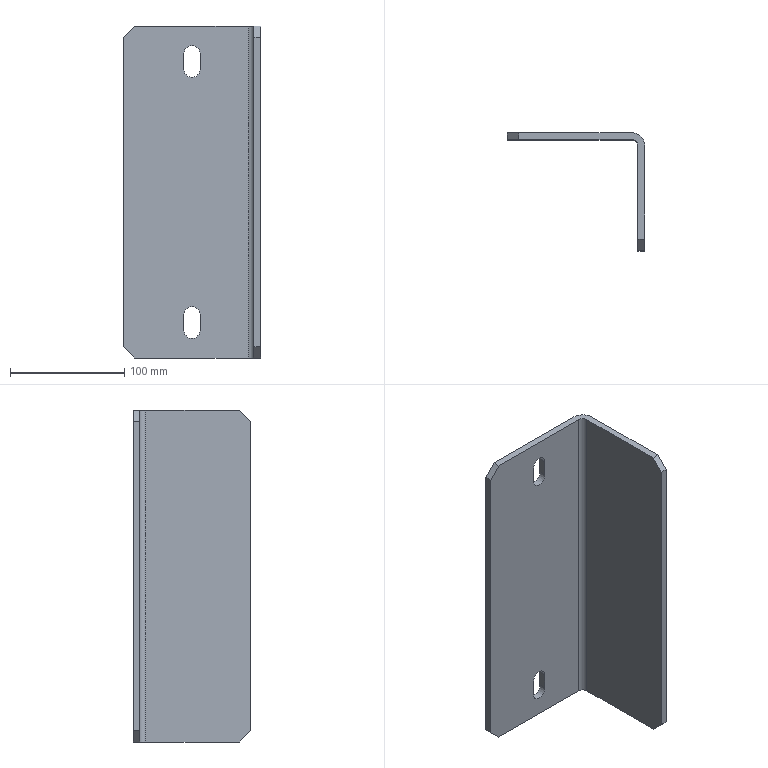Part | STEP file | VD-SYL0380DJ1006_1_1_4-2_VD-SYL | 1 solid | 24 faces | box 120 x 103 x 290 mm | volume 366206 mm3 | plane 16 | cylinder 8 | commonest cylinder face diameters 14 x6 10 x1 22 x1
STEP:
#1=CARTESIAN_POINT('',(7.,22.5,-107.));
#2=VERTEX_POINT('',#1);
#3=CARTESIAN_POINT('',(7.,22.5,-121.));
#4=VERTEX_POINT('',#3);
#5=CARTESIAN_POINT('',(7.,22.5,-107.));
#6=DIRECTION('',(0.,0.,-1.));
#7=VECTOR('',#6,1000.);
#8=LINE('',#5,#7);
#9=EDGE_CURVE('',#2,#4,#8,.T.);
#10=ORIENTED_EDGE('',*,*,#9,.T.);
#11=CARTESIAN_POINT('',(7.,16.5,-121.));
#12=VERTEX_POINT('',#11);
#13=CARTESIAN_POINT('',(7.,16.5,-121.));
#14=DIRECTION('',(0.,1.,0.));
#15=VECTOR('',#14,1000.);
#16=LINE('',#13,#15);
#17=EDGE_CURVE('',#12,#4,#16,.T.);
#18=ORIENTED_EDGE('',*,*,#17,.F.);
#19=CARTESIAN_POINT('',(7.,16.5,-107.));
#20=VERTEX_POINT('',#19);
#21=CARTESIAN_POINT('',(7.,16.5,-107.));
#22=DIRECTION('',(0.,0.,-1.));
#23=VECTOR('',#22,1000.);
#24=LINE('',#21,#23);
#25=EDGE_CURVE('',#20,#12,#24,.T.);
#26=ORIENTED_EDGE('',*,*,#25,.F.);
#27=CARTESIAN_POINT('',(7.,22.5,-107.));
#28=DIRECTION('',(0.,-1.,0.));
#29=VECTOR('',#28,1000.);
#30=LINE('',#27,#29);
#31=EDGE_CURVE('',#2,#20,#30,.T.);
#32=ORIENTED_EDGE('',*,*,#31,.F.);
#33=EDGE_LOOP('',(#10,#18,#26,#32));
#34=FACE_OUTER_BOUND('',#33,.T.);
#35=CARTESIAN_POINT('',(7.,19.5,-117.5));
#36=DIRECTION('',(-1.,0.,0.));
#37=DIRECTION('',(0.,0.,1.));
#38=AXIS2_PLACEMENT_3D('',#35,#36,#37);
#39=PLANE('',#38);
#40=ADVANCED_FACE('',(#34),#39,.T.);
#41=CARTESIAN_POINT('',(0.,22.5,-100.));
#42=VERTEX_POINT('',#41);
#43=CARTESIAN_POINT('',(0.,16.5,-100.));
#44=VERTEX_POINT('',#43);
#45=CARTESIAN_POINT('',(0.,22.5,-100.));
#46=DIRECTION('',(0.,-1.,0.));
#47=VECTOR('',#46,1000.);
#48=LINE('',#45,#47);
#49=EDGE_CURVE('',#42,#44,#48,.T.);
#50=ORIENTED_EDGE('',*,*,#49,.F.);
#51=CARTESIAN_POINT('',(0.,22.5,-107.));
#52=DIRECTION('',(0.,-1.,0.));
#53=DIRECTION('',(1.,0.,0.));
#54=AXIS2_PLACEMENT_3D('',#51,#52,#53);
#55=CIRCLE('',#54,7.);
#56=EDGE_CURVE('',#2,#42,#55,.T.);
#57=ORIENTED_EDGE('',*,*,#56,.F.);
#58=ORIENTED_EDGE('',*,*,#31,.T.);
#59=CARTESIAN_POINT('',(0.,16.5,-107.));
#60=DIRECTION('',(0.,1.,0.));
#61=DIRECTION('',(0.,0.,1.));
#62=AXIS2_PLACEMENT_3D('',#59,#60,#61);
#63=CIRCLE('',#62,7.);
#64=EDGE_CURVE('',#44,#20,#63,.T.);
#65=ORIENTED_EDGE('',*,*,#64,.F.);
#66=EDGE_LOOP('',(#50,#57,#58,#65));
#67=FACE_OUTER_BOUND('',#66,.T.);
#68=CARTESIAN_POINT('',(0.,19.5,-107.));
#69=DIRECTION('',(0.,1.,0.));
#70=DIRECTION('',(0.,0.,1.));
#71=AXIS2_PLACEMENT_3D('',#68,#69,#70);
#72=CYLINDRICAL_SURFACE('',#71,7.);
#73=ADVANCED_FACE('',(#67),#72,.F.);
#74=CARTESIAN_POINT('',(-7.,16.5,-107.));
#75=VERTEX_POINT('',#74);
#76=CARTESIAN_POINT('',(0.,16.5,-107.));
#77=DIRECTION('',(0.,1.,0.));
#78=DIRECTION('',(-1.,0.,0.));
#79=AXIS2_PLACEMENT_3D('',#76,#77,#78);
#80=CIRCLE('',#79,7.);
#81=EDGE_CURVE('',#75,#44,#80,.T.);
#82=ORIENTED_EDGE('',*,*,#81,.F.);
#83=CARTESIAN_POINT('',(-7.,22.5,-107.));
#84=VERTEX_POINT('',#83);
#85=CARTESIAN_POINT('',(-7.,16.5,-107.));
#86=DIRECTION('',(0.,1.,0.));
#87=VECTOR('',#86,1000.);
#88=LINE('',#85,#87);
#89=EDGE_CURVE('',#75,#84,#88,.T.);
#90=ORIENTED_EDGE('',*,*,#89,.T.);
#91=CARTESIAN_POINT('',(0.,22.5,-107.));
#92=DIRECTION('',(0.,-1.,0.));
#93=DIRECTION('',(0.,0.,1.));
#94=AXIS2_PLACEMENT_3D('',#91,#92,#93);
#95=CIRCLE('',#94,7.);
#96=EDGE_CURVE('',#42,#84,#95,.T.);
#97=ORIENTED_EDGE('',*,*,#96,.F.);
#98=ORIENTED_EDGE('',*,*,#49,.T.);
#99=EDGE_LOOP('',(#82,#90,#97,#98));
#100=FACE_OUTER_BOUND('',#99,.T.);
#101=CARTESIAN_POINT('',(0.,19.5,-107.));
#102=DIRECTION('',(0.,1.,0.));
#103=DIRECTION('',(0.,0.,1.));
#104=AXIS2_PLACEMENT_3D('',#101,#102,#103);
#105=CYLINDRICAL_SURFACE('',#104,7.);
#106=ADVANCED_FACE('',(#100),#105,.F.);
#107=CARTESIAN_POINT('',(-7.,22.5,-121.));
#108=VERTEX_POINT('',#107);
#109=CARTESIAN_POINT('',(-7.,22.5,-121.));
#110=DIRECTION('',(0.,0.,1.));
#111=VECTOR('',#110,1000.);
#112=LINE('',#109,#111);
#113=EDGE_CURVE('',#108,#84,#112,.T.);
#114=ORIENTED_EDGE('',*,*,#113,.T.);
#115=ORIENTED_EDGE('',*,*,#89,.F.);
#116=CARTESIAN_POINT('',(-7.,16.5,-121.));
#117=VERTEX_POINT('',#116);
#118=CARTESIAN_POINT('',(-7.,16.5,-121.));
#119=DIRECTION('',(0.,0.,1.));
#120=VECTOR('',#119,1000.);
#121=LINE('',#118,#120);
#122=EDGE_CURVE('',#117,#75,#121,.T.);
#123=ORIENTED_EDGE('',*,*,#122,.F.);
#124=CARTESIAN_POINT('',(-7.,22.5,-121.));
#125=DIRECTION('',(0.,-1.,0.));
#126=VECTOR('',#125,1000.);
#127=LINE('',#124,#126);
#128=EDGE_CURVE('',#108,#117,#127,.T.);
#129=ORIENTED_EDGE('',*,*,#128,.F.);
#130=EDGE_LOOP('',(#114,#115,#123,#129));
#131=FACE_OUTER_BOUND('',#130,.T.);
#132=CARTESIAN_POINT('',(-7.,19.5,-110.5));
#133=DIRECTION('',(1.,0.,0.));
#134=DIRECTION('',(0.,1.,0.));
#135=AXIS2_PLACEMENT_3D('',#132,#133,#134);
#136=PLANE('',#135);
#137=ADVANCED_FACE('',(#131),#136,.T.);
#138=CARTESIAN_POINT('',(-7.,16.5,121.));
#139=VERTEX_POINT('',#138);
#140=CARTESIAN_POINT('',(0.,16.5,128.));
#141=VERTEX_POINT('',#140);
#142=CARTESIAN_POINT('',(0.,16.5,121.));
#143=DIRECTION('',(0.,1.,0.));
#144=DIRECTION('',(-1.,0.,0.));
#145=AXIS2_PLACEMENT_3D('',#142,#143,#144);
#146=CIRCLE('',#145,7.);
#147=EDGE_CURVE('',#139,#141,#146,.T.);
#148=ORIENTED_EDGE('',*,*,#147,.F.);
#149=CARTESIAN_POINT('',(-7.,22.5,121.));
#150=VERTEX_POINT('',#149);
#151=CARTESIAN_POINT('',(-7.,16.5,121.));
#152=DIRECTION('',(0.,1.,0.));
#153=VECTOR('',#152,1000.);
#154=LINE('',#151,#153);
#155=EDGE_CURVE('',#139,#150,#154,.T.);
#156=ORIENTED_EDGE('',*,*,#155,.T.);
#157=CARTESIAN_POINT('',(0.,22.5,128.));
#158=VERTEX_POINT('',#157);
#159=CARTESIAN_POINT('',(0.,22.5,121.));
#160=DIRECTION('',(0.,-1.,0.));
#161=DIRECTION('',(0.,0.,1.));
#162=AXIS2_PLACEMENT_3D('',#159,#160,#161);
#163=CIRCLE('',#162,7.);
#164=EDGE_CURVE('',#158,#150,#163,.T.);
#165=ORIENTED_EDGE('',*,*,#164,.F.);
#166=CARTESIAN_POINT('',(0.,22.5,128.));
#167=DIRECTION('',(0.,-1.,0.));
#168=VECTOR('',#167,1000.);
#169=LINE('',#166,#168);
#170=EDGE_CURVE('',#158,#141,#169,.T.);
#171=ORIENTED_EDGE('',*,*,#170,.T.);
#172=EDGE_LOOP('',(#148,#156,#165,#171));
#173=FACE_OUTER_BOUND('',#172,.T.);
#174=CARTESIAN_POINT('',(0.,19.5,121.));
#175=DIRECTION('',(0.,1.,0.));
#176=DIRECTION('',(0.,0.,1.));
#177=AXIS2_PLACEMENT_3D('',#174,#175,#176);
#178=CYLINDRICAL_SURFACE('',#177,7.);
#179=ADVANCED_FACE('',(#173),#178,.F.);
#180=CARTESIAN_POINT('',(-7.,22.5,107.));
#181=VERTEX_POINT('',#180);
#182=CARTESIAN_POINT('',(-7.,22.5,107.));
#183=DIRECTION('',(0.,0.,1.));
#184=VECTOR('',#183,1000.);
#185=LINE('',#182,#184);
#186=EDGE_CURVE('',#181,#150,#185,.T.);
#187=ORIENTED_EDGE('',*,*,#186,.T.);
#188=ORIENTED_EDGE('',*,*,#155,.F.);
#189=CARTESIAN_POINT('',(-7.,16.5,107.));
#190=VERTEX_POINT('',#189);
#191=CARTESIAN_POINT('',(-7.,16.5,107.));
#192=DIRECTION('',(0.,0.,1.));
#193=VECTOR('',#192,1000.);
#194=LINE('',#191,#193);
#195=EDGE_CURVE('',#190,#139,#194,.T.);
#196=ORIENTED_EDGE('',*,*,#195,.F.);
#197=CARTESIAN_POINT('',(-7.,22.5,107.));
#198=DIRECTION('',(0.,-1.,0.));
#199=VECTOR('',#198,1000.);
#200=LINE('',#197,#199);
#201=EDGE_CURVE('',#181,#190,#200,.T.);
#202=ORIENTED_EDGE('',*,*,#201,.F.);
#203=EDGE_LOOP('',(#187,#188,#196,#202));
#204=FACE_OUTER_BOUND('',#203,.T.);
#205=CARTESIAN_POINT('',(-7.,19.5,117.5));
#206=DIRECTION('',(1.,0.,0.));
#207=DIRECTION('',(0.,1.,0.));
#208=AXIS2_PLACEMENT_3D('',#205,#206,#207);
#209=PLANE('',#208);
#210=ADVANCED_FACE('',(#204),#209,.T.);
#211=CARTESIAN_POINT('',(7.,16.5,107.));
#212=VERTEX_POINT('',#211);
#213=CARTESIAN_POINT('',(0.,16.5,107.));
#214=DIRECTION('',(0.,1.,0.));
#215=DIRECTION('',(1.,0.,0.));
#216=AXIS2_PLACEMENT_3D('',#213,#214,#215);
#217=CIRCLE('',#216,7.);
#218=EDGE_CURVE('',#212,#190,#217,.T.);
#219=ORIENTED_EDGE('',*,*,#218,.F.);
#220=CARTESIAN_POINT('',(7.,22.5,107.));
#221=VERTEX_POINT('',#220);
#222=CARTESIAN_POINT('',(7.,16.5,107.));
#223=DIRECTION('',(0.,1.,0.));
#224=VECTOR('',#223,1000.);
#225=LINE('',#222,#224);
#226=EDGE_CURVE('',#212,#221,#225,.T.);
#227=ORIENTED_EDGE('',*,*,#226,.T.);
#228=CARTESIAN_POINT('',(0.,22.5,107.));
#229=DIRECTION('',(0.,-1.,0.));
#230=DIRECTION('',(-1.,0.,0.));
#231=AXIS2_PLACEMENT_3D('',#228,#229,#230);
#232=CIRCLE('',#231,7.);
#233=EDGE_CURVE('',#181,#221,#232,.T.);
#234=ORIENTED_EDGE('',*,*,#233,.F.);
#235=ORIENTED_EDGE('',*,*,#201,.T.);
#236=EDGE_LOOP('',(#219,#227,#234,#235));
#237=FACE_OUTER_BOUND('',#236,.T.);
#238=CARTESIAN_POINT('',(0.,19.5,107.));
#239=DIRECTION('',(0.,1.,0.));
#240=DIRECTION('',(0.,0.,1.));
#241=AXIS2_PLACEMENT_3D('',#238,#239,#240);
#242=CYLINDRICAL_SURFACE('',#241,7.);
#243=ADVANCED_FACE('',(#237),#242,.F.);
#244=CARTESIAN_POINT('',(7.,22.5,121.));
#245=VERTEX_POINT('',#244);
#246=CARTESIAN_POINT('',(7.,22.5,121.));
#247=DIRECTION('',(0.,0.,-1.));
#248=VECTOR('',#247,1000.);
#249=LINE('',#246,#248);
#250=EDGE_CURVE('',#245,#221,#249,.T.);
#251=ORIENTED_EDGE('',*,*,#250,.T.);
#252=ORIENTED_EDGE('',*,*,#226,.F.);
#253=CARTESIAN_POINT('',(7.,16.5,121.));
#254=VERTEX_POINT('',#253);
#255=CARTESIAN_POINT('',(7.,16.5,121.));
#256=DIRECTION('',(0.,0.,-1.));
#257=VECTOR('',#256,1000.);
#258=LINE('',#255,#257);
#259=EDGE_CURVE('',#254,#212,#258,.T.);
#260=ORIENTED_EDGE('',*,*,#259,.F.);
#261=CARTESIAN_POINT('',(7.,22.5,121.));
#262=DIRECTION('',(0.,-1.,0.));
#263=VECTOR('',#262,1000.);
#264=LINE('',#261,#263);
#265=EDGE_CURVE('',#245,#254,#264,.T.);
#266=ORIENTED_EDGE('',*,*,#265,.F.);
#267=EDGE_LOOP('',(#251,#252,#260,#266));
#268=FACE_OUTER_BOUND('',#267,.T.);
#269=CARTESIAN_POINT('',(7.,19.5,110.5));
#270=DIRECTION('',(-1.,0.,0.));
#271=DIRECTION('',(0.,0.,1.));
#272=AXIS2_PLACEMENT_3D('',#269,#270,#271);
#273=PLANE('',#272);
#274=ADVANCED_FACE('',(#268),#273,.T.);
#275=ORIENTED_EDGE('',*,*,#170,.F.);
#276=CARTESIAN_POINT('',(0.,22.5,121.));
#277=DIRECTION('',(0.,-1.,0.));
#278=DIRECTION('',(1.,0.,0.));
#279=AXIS2_PLACEMENT_3D('',#276,#277,#278);
#280=CIRCLE('',#279,7.);
#281=EDGE_CURVE('',#245,#158,#280,.T.);
#282=ORIENTED_EDGE('',*,*,#281,.F.);
#283=ORIENTED_EDGE('',*,*,#265,.T.);
#284=CARTESIAN_POINT('',(0.,16.5,121.));
#285=DIRECTION('',(0.,1.,0.));
#286=DIRECTION('',(0.,0.,1.));
#287=AXIS2_PLACEMENT_3D('',#284,#285,#286);
#288=CIRCLE('',#287,7.);
#289=EDGE_CURVE('',#141,#254,#288,.T.);
#290=ORIENTED_EDGE('',*,*,#289,.F.);
#291=EDGE_LOOP('',(#275,#282,#283,#290));
#292=FACE_OUTER_BOUND('',#291,.T.);
#293=CARTESIAN_POINT('',(0.,19.5,121.));
#294=DIRECTION('',(0.,1.,0.));
#295=DIRECTION('',(0.,0.,1.));
#296=AXIS2_PLACEMENT_3D('',#293,#294,#295);
#297=CYLINDRICAL_SURFACE('',#296,7.);
#298=ADVANCED_FACE('',(#292),#297,.F.);
#299=CARTESIAN_POINT('',(-50.,22.5,-145.));
#300=VERTEX_POINT('',#299);
#301=CARTESIAN_POINT('',(-60.,22.5,-135.));
#302=VERTEX_POINT('',#301);
#303=CARTESIAN_POINT('',(-50.,22.5,-145.));
#304=DIRECTION('',(-0.7071,0.,0.7071));
#305=VECTOR('',#304,1000.);
#306=LINE('',#303,#305);
#307=EDGE_CURVE('',#300,#302,#306,.T.);
#308=ORIENTED_EDGE('',*,*,#307,.F.);
#309=CARTESIAN_POINT('',(-50.,16.5,-145.));
#310=VERTEX_POINT('',#309);
#311=CARTESIAN_POINT('',(-50.,16.5,-145.));
#312=DIRECTION('',(0.,1.,0.));
#313=VECTOR('',#312,1000.);
#314=LINE('',#311,#313);
#315=EDGE_CURVE('',#310,#300,#314,.T.);
#316=ORIENTED_EDGE('',*,*,#315,.F.);
#317=CARTESIAN_POINT('',(-60.,16.5,-135.));
#318=VERTEX_POINT('',#317);
#319=CARTESIAN_POINT('',(-60.,16.5,-135.));
#320=DIRECTION('',(0.7071,0.,-0.7071));
#321=VECTOR('',#320,1000.);
#322=LINE('',#319,#321);
#323=EDGE_CURVE('',#318,#310,#322,.T.);
#324=ORIENTED_EDGE('',*,*,#323,.F.);
#325=CARTESIAN_POINT('',(-60.,22.5,-135.));
#326=DIRECTION('',(0.,-1.,0.));
#327=VECTOR('',#326,1000.);
#328=LINE('',#325,#327);
#329=EDGE_CURVE('',#302,#318,#328,.T.);
#330=ORIENTED_EDGE('',*,*,#329,.F.);
#331=EDGE_LOOP('',(#308,#316,#324,#330));
#332=FACE_OUTER_BOUND('',#331,.T.);
#333=CARTESIAN_POINT('',(-55.,19.5,-140.));
#334=DIRECTION('',(-0.7071,0.,-0.7071));
#335=DIRECTION('',(-0.7071,0.,0.7071));
#336=AXIS2_PLACEMENT_3D('',#333,#334,#335);
#337=PLANE('',#336);
#338=ADVANCED_FACE('',(#332),#337,.T.);
#339=CARTESIAN_POINT('',(60.,11.5,145.));
#340=VERTEX_POINT('',#339);
#341=CARTESIAN_POINT('',(60.,11.5,-145.));
#342=VERTEX_POINT('',#341);
#343=CARTESIAN_POINT('',(60.,11.5,145.));
#344=DIRECTION('',(0.,0.,-1.));
#345=VECTOR('',#344,1000.);
#346=LINE('',#343,#345);
#347=EDGE_CURVE('',#340,#342,#346,.T.);
#348=ORIENTED_EDGE('',*,*,#347,.T.);
#349=CARTESIAN_POINT('',(49.,22.5,-145.));
#350=VERTEX_POINT('',#349);
#351=CARTESIAN_POINT('',(49.,11.5,-145.));
#352=DIRECTION('',(0.,0.,-1.));
#353=DIRECTION('',(0.,1.,0.));
#354=AXIS2_PLACEMENT_3D('',#351,#352,#353);
#355=CIRCLE('',#354,11.);
#356=EDGE_CURVE('',#350,#342,#355,.T.);
#357=ORIENTED_EDGE('',*,*,#356,.F.);
#358=CARTESIAN_POINT('',(49.,22.5,145.));
#359=VERTEX_POINT('',#358);
#360=CARTESIAN_POINT('',(49.,22.5,-145.));
#361=DIRECTION('',(0.,0.,1.));
#362=VECTOR('',#361,1000.);
#363=LINE('',#360,#362);
#364=EDGE_CURVE('',#350,#359,#363,.T.);
#365=ORIENTED_EDGE('',*,*,#364,.T.);
#366=CARTESIAN_POINT('',(49.,11.5,145.));
#367=DIRECTION('',(0.,0.,1.));
#368=DIRECTION('',(1.,0.,0.));
#369=AXIS2_PLACEMENT_3D('',#366,#367,#368);
#370=CIRCLE('',#369,11.);
#371=EDGE_CURVE('',#340,#359,#370,.T.);
#372=ORIENTED_EDGE('',*,*,#371,.F.);
#373=EDGE_LOOP('',(#348,#357,#365,#372));
#374=FACE_OUTER_BOUND('',#373,.T.);
#375=CARTESIAN_POINT('',(49.,11.5,523.044));
#376=DIRECTION('',(0.,0.,-1.));
#377=DIRECTION('',(-1.,0.,0.));
#378=AXIS2_PLACEMENT_3D('',#375,#376,#377);
#379=CYLINDRICAL_SURFACE('',#378,11.);
#380=ADVANCED_FACE('',(#374),#379,.T.);
#381=CARTESIAN_POINT('',(60.,-70.5,145.));
#382=VERTEX_POINT('',#381);
#383=CARTESIAN_POINT('',(60.,-80.5,135.));
#384=VERTEX_POINT('',#383);
#385=CARTESIAN_POINT('',(60.,-70.5,145.));
#386=DIRECTION('',(0.,-0.7071,-0.7071));
#387=VECTOR('',#386,1000.);
#388=LINE('',#385,#387);
#389=EDGE_CURVE('',#382,#384,#388,.T.);
#390=ORIENTED_EDGE('',*,*,#389,.T.);
#391=CARTESIAN_POINT('',(60.,-80.5,-135.));
#392=VERTEX_POINT('',#391);
#393=CARTESIAN_POINT('',(60.,-80.5,-135.));
#394=DIRECTION('',(0.,0.,1.));
#395=VECTOR('',#394,1000.);
#396=LINE('',#393,#395);
#397=EDGE_CURVE('',#392,#384,#396,.T.);
#398=ORIENTED_EDGE('',*,*,#397,.F.);
#399=CARTESIAN_POINT('',(60.,-70.5,-145.));
#400=VERTEX_POINT('',#399);
#401=CARTESIAN_POINT('',(60.,-80.5,-135.));
#402=DIRECTION('',(0.,0.7071,-0.7071));
#403=VECTOR('',#402,1000.);
#404=LINE('',#401,#403);
#405=EDGE_CURVE('',#392,#400,#404,.T.);
#406=ORIENTED_EDGE('',*,*,#405,.T.);
#407=CARTESIAN_POINT('',(60.,11.5,-145.));
#408=DIRECTION('',(0.,-1.,0.));
#409=VECTOR('',#408,1000.);
#410=LINE('',#407,#409);
#411=EDGE_CURVE('',#342,#400,#410,.T.);
#412=ORIENTED_EDGE('',*,*,#411,.F.);
#413=ORIENTED_EDGE('',*,*,#347,.F.);
#414=CARTESIAN_POINT('',(60.,-70.5,145.));
#415=DIRECTION('',(0.,1.,0.));
#416=VECTOR('',#415,1000.);
#417=LINE('',#414,#416);
#418=EDGE_CURVE('',#382,#340,#417,.T.);
#419=ORIENTED_EDGE('',*,*,#418,.F.);
#420=EDGE_LOOP('',(#390,#398,#406,#412,#413,#419));
#421=FACE_OUTER_BOUND('',#420,.T.);
#422=CARTESIAN_POINT('',(60.,-80.5,-145.));
#423=DIRECTION('',(1.,0.,0.));
#424=DIRECTION('',(0.,1.,0.));
#425=AXIS2_PLACEMENT_3D('',#422,#423,#424);
#426=PLANE('',#425);
#427=ADVANCED_FACE('',(#421),#426,.T.);
#428=ORIENTED_EDGE('',*,*,#405,.F.);
#429=CARTESIAN_POINT('',(54.,-80.5,-135.));
#430=VERTEX_POINT('',#429);
#431=CARTESIAN_POINT('',(54.,-80.5,-135.));
#432=DIRECTION('',(1.,0.,0.));
#433=VECTOR('',#432,1000.);
#434=LINE('',#431,#433);
#435=EDGE_CURVE('',#430,#392,#434,.T.);
#436=ORIENTED_EDGE('',*,*,#435,.F.);
#437=CARTESIAN_POINT('',(54.,-70.5,-145.));
#438=VERTEX_POINT('',#437);
#439=CARTESIAN_POINT('',(54.,-70.5,-145.));
#440=DIRECTION('',(0.,-0.7071,0.7071));
#441=VECTOR('',#440,1000.);
#442=LINE('',#439,#441);
#443=EDGE_CURVE('',#438,#430,#442,.T.);
#444=ORIENTED_EDGE('',*,*,#443,.F.);
#445=CARTESIAN_POINT('',(54.,-70.5,-145.));
#446=DIRECTION('',(1.,0.,0.));
#447=VECTOR('',#446,1000.);
#448=LINE('',#445,#447);
#449=EDGE_CURVE('',#438,#400,#448,.T.);
#450=ORIENTED_EDGE('',*,*,#449,.T.);
#451=EDGE_LOOP('',(#428,#436,#444,#450));
#452=FACE_OUTER_BOUND('',#451,.T.);
#453=CARTESIAN_POINT('',(57.,-75.5,-140.));
#454=DIRECTION('',(0.,-0.7071,-0.7071));
#455=DIRECTION('',(0.,-0.7071,0.7071));
#456=AXIS2_PLACEMENT_3D('',#453,#454,#455);
#457=PLANE('',#456);
#458=ADVANCED_FACE('',(#452),#457,.T.);
#459=ORIENTED_EDGE('',*,*,#397,.T.);
#460=CARTESIAN_POINT('',(54.,-80.5,135.));
#461=VERTEX_POINT('',#460);
#462=CARTESIAN_POINT('',(60.,-80.5,135.));
#463=DIRECTION('',(-1.,0.,0.));
#464=VECTOR('',#463,1000.);
#465=LINE('',#462,#464);
#466=EDGE_CURVE('',#384,#461,#465,.T.);
#467=ORIENTED_EDGE('',*,*,#466,.T.);
#468=CARTESIAN_POINT('',(54.,-80.5,135.));
#469=DIRECTION('',(0.,0.,-1.));
#470=VECTOR('',#469,1000.);
#471=LINE('',#468,#470);
#472=EDGE_CURVE('',#461,#430,#471,.T.);
#473=ORIENTED_EDGE('',*,*,#472,.T.);
#474=ORIENTED_EDGE('',*,*,#435,.T.);
#475=EDGE_LOOP('',(#459,#467,#473,#474));
#476=FACE_OUTER_BOUND('',#475,.T.);
#477=CARTESIAN_POINT('',(57.,-80.5,0.));
#478=DIRECTION('',(0.,1.,0.));
#479=DIRECTION('',(1.,0.,0.));
#480=AXIS2_PLACEMENT_3D('',#477,#478,#479);
#481=PLANE('',#480);
#482=ADVANCED_FACE('',(#476),#481,.F.);
#483=ORIENTED_EDGE('',*,*,#389,.F.);
#484=CARTESIAN_POINT('',(54.,-70.5,145.));
#485=VERTEX_POINT('',#484);
#486=CARTESIAN_POINT('',(54.,-70.5,145.));
#487=DIRECTION('',(1.,0.,0.));
#488=VECTOR('',#487,1000.);
#489=LINE('',#486,#488);
#490=EDGE_CURVE('',#485,#382,#489,.T.);
#491=ORIENTED_EDGE('',*,*,#490,.F.);
#492=CARTESIAN_POINT('',(54.,-80.5,135.));
#493=DIRECTION('',(0.,0.7071,0.7071));
#494=VECTOR('',#493,1000.);
#495=LINE('',#492,#494);
#496=EDGE_CURVE('',#461,#485,#495,.T.);
#497=ORIENTED_EDGE('',*,*,#496,.F.);
#498=ORIENTED_EDGE('',*,*,#466,.F.);
#499=EDGE_LOOP('',(#483,#491,#497,#498));
#500=FACE_OUTER_BOUND('',#499,.T.);
#501=CARTESIAN_POINT('',(57.,-75.5,140.));
#502=DIRECTION('',(0.,-0.7071,0.7071));
#503=DIRECTION('',(-1.,0.,0.));
#504=AXIS2_PLACEMENT_3D('',#501,#502,#503);
#505=PLANE('',#504);
#506=ADVANCED_FACE('',(#500),#505,.T.);
#507=CARTESIAN_POINT('',(54.,11.5,-145.));
#508=VERTEX_POINT('',#507);
#509=CARTESIAN_POINT('',(54.,11.5,-145.));
#510=DIRECTION('',(0.,-1.,0.));
#511=VECTOR('',#510,1000.);
#512=LINE('',#509,#511);
#513=EDGE_CURVE('',#508,#438,#512,.T.);
#514=ORIENTED_EDGE('',*,*,#513,.T.);
#515=ORIENTED_EDGE('',*,*,#443,.T.);
#516=ORIENTED_EDGE('',*,*,#472,.F.);
#517=ORIENTED_EDGE('',*,*,#496,.T.);
#518=CARTESIAN_POINT('',(54.,11.5,145.));
#519=VERTEX_POINT('',#518);
#520=CARTESIAN_POINT('',(54.,11.5,145.));
#521=DIRECTION('',(0.,-1.,0.));
#522=VECTOR('',#521,1000.);
#523=LINE('',#520,#522);
#524=EDGE_CURVE('',#519,#485,#523,.T.);
#525=ORIENTED_EDGE('',*,*,#524,.F.);
#526=CARTESIAN_POINT('',(54.,11.5,-145.));
#527=DIRECTION('',(0.,0.,1.));
#528=VECTOR('',#527,1000.);
#529=LINE('',#526,#528);
#530=EDGE_CURVE('',#508,#519,#529,.T.);
#531=ORIENTED_EDGE('',*,*,#530,.F.);
#532=EDGE_LOOP('',(#514,#515,#516,#517,#525,#531));
#533=FACE_OUTER_BOUND('',#532,.T.);
#534=CARTESIAN_POINT('',(54.,-80.5,-145.));
#535=DIRECTION('',(1.,0.,0.));
#536=DIRECTION('',(0.,1.,0.));
#537=AXIS2_PLACEMENT_3D('',#534,#535,#536);
#538=PLANE('',#537);
#539=ADVANCED_FACE('',(#533),#538,.F.);
#540=ORIENTED_EDGE('',*,*,#315,.T.);
#541=CARTESIAN_POINT('',(-50.,22.5,-145.));
#542=DIRECTION('',(1.,0.,0.));
#543=VECTOR('',#542,1000.);
#544=LINE('',#541,#543);
#545=EDGE_CURVE('',#300,#350,#544,.T.);
#546=ORIENTED_EDGE('',*,*,#545,.T.);
#547=ORIENTED_EDGE('',*,*,#356,.T.);
#548=ORIENTED_EDGE('',*,*,#411,.T.);
#549=ORIENTED_EDGE('',*,*,#449,.F.);
#550=ORIENTED_EDGE('',*,*,#513,.F.);
#551=CARTESIAN_POINT('',(49.,16.5,-145.));
#552=VERTEX_POINT('',#551);
#553=CARTESIAN_POINT('',(49.,11.5,-145.));
#554=DIRECTION('',(0.,0.,1.));
#555=DIRECTION('',(1.,0.,0.));
#556=AXIS2_PLACEMENT_3D('',#553,#554,#555);
#557=CIRCLE('',#556,5.);
#558=EDGE_CURVE('',#508,#552,#557,.T.);
#559=ORIENTED_EDGE('',*,*,#558,.T.);
#560=CARTESIAN_POINT('',(-50.,16.5,-145.));
#561=DIRECTION('',(1.,0.,0.));
#562=VECTOR('',#561,1000.);
#563=LINE('',#560,#562);
#564=EDGE_CURVE('',#310,#552,#563,.T.);
#565=ORIENTED_EDGE('',*,*,#564,.F.);
#566=EDGE_LOOP('',(#540,#546,#547,#548,#549,#550,#559,#565));
#567=FACE_OUTER_BOUND('',#566,.T.);
#568=CARTESIAN_POINT('',(-1.5,19.5,-145.));
#569=DIRECTION('',(0.,0.,-1.));
#570=DIRECTION('',(0.,-1.,0.));
#571=AXIS2_PLACEMENT_3D('',#568,#569,#570);
#572=PLANE('',#571);
#573=ADVANCED_FACE('',(#567),#572,.T.);
#574=ORIENTED_EDGE('',*,*,#113,.F.);
#575=CARTESIAN_POINT('',(0.,22.5,-121.));
#576=DIRECTION('',(0.,-1.,0.));
#577=DIRECTION('',(0.,0.,-1.));
#578=AXIS2_PLACEMENT_3D('',#575,#576,#577);
#579=CIRCLE('',#578,7.);
#580=EDGE_CURVE('',#108,#4,#579,.T.);
#581=ORIENTED_EDGE('',*,*,#580,.T.);
#582=ORIENTED_EDGE('',*,*,#9,.F.);
#583=ORIENTED_EDGE('',*,*,#56,.T.);
#584=ORIENTED_EDGE('',*,*,#96,.T.);
#585=EDGE_LOOP('',(#574,#581,#582,#583,#584));
#586=FACE_BOUND('',#585,.T.);
#587=ORIENTED_EDGE('',*,*,#164,.T.);
#588=ORIENTED_EDGE('',*,*,#186,.F.);
#589=ORIENTED_EDGE('',*,*,#233,.T.);
#590=ORIENTED_EDGE('',*,*,#250,.F.);
#591=ORIENTED_EDGE('',*,*,#281,.T.);
#592=EDGE_LOOP('',(#587,#588,#589,#590,#591));
#593=FACE_BOUND('',#592,.T.);
#594=ORIENTED_EDGE('',*,*,#307,.T.);
#595=CARTESIAN_POINT('',(-60.,22.5,135.));
#596=VERTEX_POINT('',#595);
#597=CARTESIAN_POINT('',(-60.,22.5,135.));
#598=DIRECTION('',(0.,0.,-1.));
#599=VECTOR('',#598,1000.);
#600=LINE('',#597,#599);
#601=EDGE_CURVE('',#596,#302,#600,.T.);
#602=ORIENTED_EDGE('',*,*,#601,.F.);
#603=CARTESIAN_POINT('',(-50.,22.5,145.));
#604=VERTEX_POINT('',#603);
#605=CARTESIAN_POINT('',(-60.,22.5,135.));
#606=DIRECTION('',(0.7071,0.,0.7071));
#607=VECTOR('',#606,1000.);
#608=LINE('',#605,#607);
#609=EDGE_CURVE('',#596,#604,#608,.T.);
#610=ORIENTED_EDGE('',*,*,#609,.T.);
#611=CARTESIAN_POINT('',(49.,22.5,145.));
#612=DIRECTION('',(-1.,0.,0.));
#613=VECTOR('',#612,1000.);
#614=LINE('',#611,#613);
#615=EDGE_CURVE('',#359,#604,#614,.T.);
#616=ORIENTED_EDGE('',*,*,#615,.F.);
#617=ORIENTED_EDGE('',*,*,#364,.F.);
#618=ORIENTED_EDGE('',*,*,#545,.F.);
#619=EDGE_LOOP('',(#594,#602,#610,#616,#617,#618));
#620=FACE_OUTER_BOUND('',#619,.T.);
#621=CARTESIAN_POINT('',(60.,22.5,-145.));
#622=DIRECTION('',(0.,1.,0.));
#623=DIRECTION('',(1.,0.,0.));
#624=AXIS2_PLACEMENT_3D('',#621,#622,#623);
#625=PLANE('',#624);
#626=ADVANCED_FACE('',(#586,#593,#620),#625,.T.);
#627=ORIENTED_EDGE('',*,*,#329,.T.);
#628=CARTESIAN_POINT('',(-60.,16.5,135.));
#629=VERTEX_POINT('',#628);
#630=CARTESIAN_POINT('',(-60.,16.5,135.));
#631=DIRECTION('',(0.,0.,-1.));
#632=VECTOR('',#631,1000.);
#633=LINE('',#630,#632);
#634=EDGE_CURVE('',#629,#318,#633,.T.);
#635=ORIENTED_EDGE('',*,*,#634,.F.);
#636=CARTESIAN_POINT('',(-60.,16.5,135.));
#637=DIRECTION('',(0.,1.,0.));
#638=VECTOR('',#637,1000.);
#639=LINE('',#636,#638);
#640=EDGE_CURVE('',#629,#596,#639,.T.);
#641=ORIENTED_EDGE('',*,*,#640,.T.);
#642=ORIENTED_EDGE('',*,*,#601,.T.);
#643=EDGE_LOOP('',(#627,#635,#641,#642));
#644=FACE_OUTER_BOUND('',#643,.T.);
#645=CARTESIAN_POINT('',(-60.,19.5,0.));
#646=DIRECTION('',(-1.,0.,0.));
#647=DIRECTION('',(0.,0.,1.));
#648=AXIS2_PLACEMENT_3D('',#645,#646,#647);
#649=PLANE('',#648);
#650=ADVANCED_FACE('',(#644),#649,.T.);
#651=ORIENTED_EDGE('',*,*,#609,.F.);
#652=ORIENTED_EDGE('',*,*,#640,.F.);
#653=CARTESIAN_POINT('',(-50.,16.5,145.));
#654=VERTEX_POINT('',#653);
#655=CARTESIAN_POINT('',(-50.,16.5,145.));
#656=DIRECTION('',(-0.7071,0.,-0.7071));
#657=VECTOR('',#656,1000.);
#658=LINE('',#655,#657);
#659=EDGE_CURVE('',#654,#629,#658,.T.);
#660=ORIENTED_EDGE('',*,*,#659,.F.);
#661=CARTESIAN_POINT('',(-50.,22.5,145.));
#662=DIRECTION('',(0.,-1.,0.));
#663=VECTOR('',#662,1000.);
#664=LINE('',#661,#663);
#665=EDGE_CURVE('',#604,#654,#664,.T.);
#666=ORIENTED_EDGE('',*,*,#665,.F.);
#667=EDGE_LOOP('',(#651,#652,#660,#666));
#668=FACE_OUTER_BOUND('',#667,.T.);
#669=CARTESIAN_POINT('',(-55.,19.5,140.));
#670=DIRECTION('',(-0.7071,0.,0.7071));
#671=DIRECTION('',(0.,1.,0.));
#672=AXIS2_PLACEMENT_3D('',#669,#670,#671);
#673=PLANE('',#672);
#674=ADVANCED_FACE('',(#668),#673,.T.);
#675=CARTESIAN_POINT('',(49.,16.5,145.));
#676=VERTEX_POINT('',#675);
#677=CARTESIAN_POINT('',(49.,11.5,145.));
#678=DIRECTION('',(0.,0.,-1.));
#679=DIRECTION('',(0.,1.,0.));
#680=AXIS2_PLACEMENT_3D('',#677,#678,#679);
#681=CIRCLE('',#680,5.);
#682=EDGE_CURVE('',#676,#519,#681,.T.);
#683=ORIENTED_EDGE('',*,*,#682,.T.);
#684=ORIENTED_EDGE('',*,*,#524,.T.);
#685=ORIENTED_EDGE('',*,*,#490,.T.);
#686=ORIENTED_EDGE('',*,*,#418,.T.);
#687=ORIENTED_EDGE('',*,*,#371,.T.);
#688=ORIENTED_EDGE('',*,*,#615,.T.);
#689=ORIENTED_EDGE('',*,*,#665,.T.);
#690=CARTESIAN_POINT('',(-50.,16.5,145.));
#691=DIRECTION('',(1.,0.,0.));
#692=VECTOR('',#691,1000.);
#693=LINE('',#690,#692);
#694=EDGE_CURVE('',#654,#676,#693,.T.);
#695=ORIENTED_EDGE('',*,*,#694,.T.);
#696=EDGE_LOOP('',(#683,#684,#685,#686,#687,#688,#689,#695));
#697=FACE_OUTER_BOUND('',#696,.T.);
#698=CARTESIAN_POINT('',(-1.5,19.5,145.));
#699=DIRECTION('',(0.,0.,-1.));
#700=DIRECTION('',(0.,-1.,0.));
#701=AXIS2_PLACEMENT_3D('',#698,#699,#700);
#702=PLANE('',#701);
#703=ADVANCED_FACE('',(#697),#702,.F.);
#704=ORIENTED_EDGE('',*,*,#558,.F.);
#705=ORIENTED_EDGE('',*,*,#530,.T.);
#706=ORIENTED_EDGE('',*,*,#682,.F.);
#707=CARTESIAN_POINT('',(49.,16.5,145.));
#708=DIRECTION('',(0.,0.,-1.));
#709=VECTOR('',#708,1000.);
#710=LINE('',#707,#709);
#711=EDGE_CURVE('',#676,#552,#710,.T.);
#712=ORIENTED_EDGE('',*,*,#711,.T.);
#713=EDGE_LOOP('',(#704,#705,#706,#712));
#714=FACE_OUTER_BOUND('',#713,.T.);
#715=CARTESIAN_POINT('',(49.,11.5,523.044));
#716=DIRECTION('',(0.,0.,-1.));
#717=DIRECTION('',(-1.,0.,0.));
#718=AXIS2_PLACEMENT_3D('',#715,#716,#717);
#719=CYLINDRICAL_SURFACE('',#718,5.);
#720=ADVANCED_FACE('',(#714),#719,.F.);
#721=ORIENTED_EDGE('',*,*,#218,.T.);
#722=ORIENTED_EDGE('',*,*,#195,.T.);
#723=ORIENTED_EDGE('',*,*,#147,.T.);
#724=ORIENTED_EDGE('',*,*,#289,.T.);
#725=ORIENTED_EDGE('',*,*,#259,.T.);
#726=EDGE_LOOP('',(#721,#722,#723,#724,#725));
#727=FACE_BOUND('',#726,.T.);
#728=ORIENTED_EDGE('',*,*,#64,.T.);
#729=ORIENTED_EDGE('',*,*,#25,.T.);
#730=CARTESIAN_POINT('',(0.,16.5,-121.));
#731=DIRECTION('',(0.,1.,0.));
#732=DIRECTION('',(1.,0.,0.));
#733=AXIS2_PLACEMENT_3D('',#730,#731,#732);
#734=CIRCLE('',#733,7.);
#735=EDGE_CURVE('',#12,#117,#734,.T.);
#736=ORIENTED_EDGE('',*,*,#735,.T.);
#737=ORIENTED_EDGE('',*,*,#122,.T.);
#738=ORIENTED_EDGE('',*,*,#81,.T.);
#739=EDGE_LOOP('',(#728,#729,#736,#737,#738));
#740=FACE_BOUND('',#739,.T.);
#741=ORIENTED_EDGE('',*,*,#694,.F.);
#742=ORIENTED_EDGE('',*,*,#659,.T.);
#743=ORIENTED_EDGE('',*,*,#634,.T.);
#744=ORIENTED_EDGE('',*,*,#323,.T.);
#745=ORIENTED_EDGE('',*,*,#564,.T.);
#746=ORIENTED_EDGE('',*,*,#711,.F.);
#747=EDGE_LOOP('',(#741,#742,#743,#744,#745,#746));
#748=FACE_OUTER_BOUND('',#747,.T.);
#749=CARTESIAN_POINT('',(60.,16.5,-145.));
#750=DIRECTION('',(0.,1.,0.));
#751=DIRECTION('',(1.,0.,0.));
#752=AXIS2_PLACEMENT_3D('',#749,#750,#751);
#753=PLANE('',#752);
#754=ADVANCED_FACE('',(#727,#740,#748),#753,.F.);
#755=ORIENTED_EDGE('',*,*,#735,.F.);
#756=ORIENTED_EDGE('',*,*,#17,.T.);
#757=ORIENTED_EDGE('',*,*,#580,.F.);
#758=ORIENTED_EDGE('',*,*,#128,.T.);
#759=EDGE_LOOP('',(#755,#756,#757,#758));
#760=FACE_OUTER_BOUND('',#759,.T.);
#761=CARTESIAN_POINT('',(0.,19.5,-121.));
#762=DIRECTION('',(0.,1.,0.));
#763=DIRECTION('',(0.,0.,1.));
#764=AXIS2_PLACEMENT_3D('',#761,#762,#763);
#765=CYLINDRICAL_SURFACE('',#764,7.);
#766=ADVANCED_FACE('',(#760),#765,.F.);
#767=CLOSED_SHELL('',(#40,#73,#106,#137,#179,#210,#243,#274,#298,#338,#380,#427,#458,#482,#506,#539,#573,#626,#650,#674,#703,#720,#754,#766));
#768=MANIFOLD_SOLID_BREP('',#767);
#769=CARTESIAN_POINT('',(0.,0.,0.));
#770=DIRECTION('',(0.,0.,1.));
#771=DIRECTION('',(1.,0.,0.));
#772=AXIS2_PLACEMENT_3D('',#769,#770,#771);
#773=(LENGTH_UNIT()NAMED_UNIT(*)SI_UNIT(.MILLI.,.METRE.));
#774=UNCERTAINTY_MEASURE_WITH_UNIT(LENGTH_MEASURE(0.00001),#773,'','');
#775=(NAMED_UNIT(*)PLANE_ANGLE_UNIT()SI_UNIT($,.RADIAN.));
#776=(NAMED_UNIT(*)SI_UNIT($,.STERADIAN.)SOLID_ANGLE_UNIT());
#777=(GEOMETRIC_REPRESENTATION_CONTEXT(3)GLOBAL_UNCERTAINTY_ASSIGNED_CONTEXT((#774))GLOBAL_UNIT_ASSIGNED_CONTEXT((#773,#775,#776))REPRESENTATION_CONTEXT('',''));
#778=ADVANCED_BREP_SHAPE_REPRESENTATION('',(#768,#772),#777);